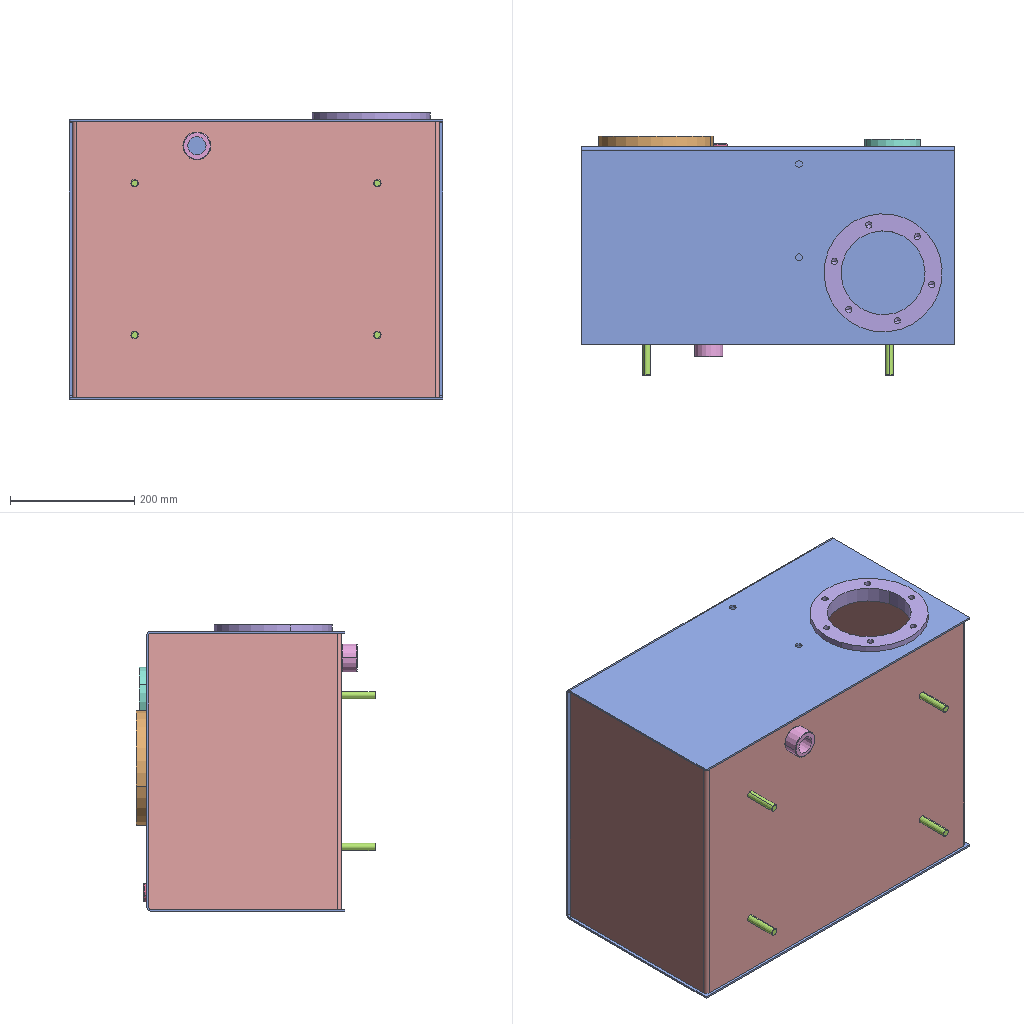Assembly | SolidWorks | 10 different items | 19 placed | box 600 x 385 x 460 mm
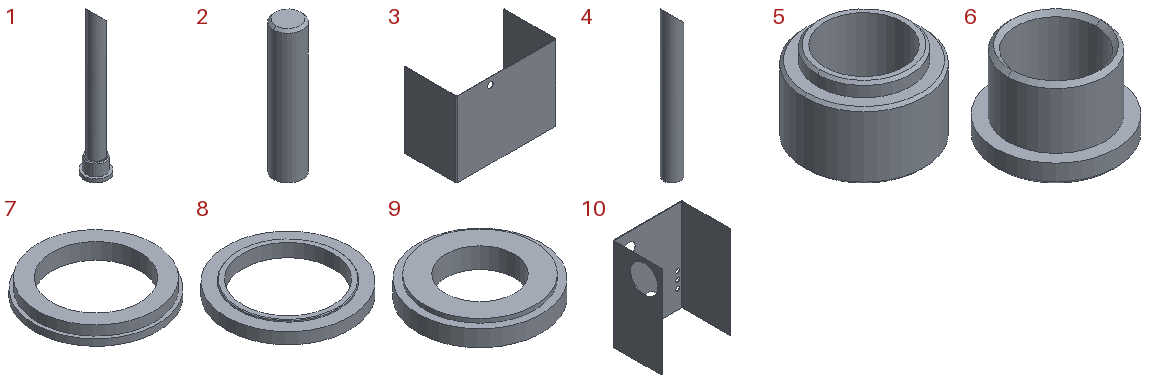Parts list (item | name | quantity | parent item | size | volume | features):
1 | (subassembly) | x3 | - | 30 x 30 x 180 mm | 11987 mm3 | features CompositeCurve 2, AEMSimFeature 1
2 | - | x4 | - | 12 x 12 x 55 mm | 6203 mm3 | features Chamfer 1, Extrusion 1
3 | - | x1 | - | 590 x 310 x 444 mm | 1595673 mm3 | features ICE 2, FlatPattern 1, SMBaseFlange 1, SheetMetal 1
4 | - | x3 | in 1 | 18 x 18 x 160 mm | 8065 mm3 | features Extrusion 1, ICE 1
5 | - | x1 | - | 45 x 45 x 30 mm | 23873 mm3 | features Chamfer 1, Extrusion 1, ICE 1
6 | - | x3 | in 1 | 30 x 30 x 20 mm | 3922 mm3 | features Chamfer 1, Extrusion 1, ICE 1
7 | - | x1 | - | 190 x 190 x 25 mm | 301982 mm3 | features 3DProfileFeature 1, Extrusion 1, HoleWzd 1, ICE 1
8 | - | x1 | - | 185 x 185 x 20 mm | 216002 mm3 | features Fillet 2, ICE 2, 3DProfileFeature 1, Chamfer 1, Extrusion 1, HoleWzd 1
9 | - | x1 | - | 90 x 90 x 15 mm | 61433 mm3 | features 3DProfileFeature 1, Extrusion 1, HoleWzd 1, ICE 1
10 | - | x1 | - | 450 x 318 x 600 mm | 1787947 mm3 | features ICE 3, FlatPattern 1, SMBaseFlange 1, SheetMetal 1
Mates (type | each side: item.copy, entity, surface, feature):
In the top assembly
Coincident | 3.1 face plane Base-Flange1 | 10.1 face plane Base-Flange1 | 2 times
DistanceDim | 10.1 face plane Base-Flange1 | 3.1 face plane Base-Flange1
Concentric | 2.1 edge | assembly select_type:10
Coincident | 3.1 face plane Base-Flange1 | 2.1 face plane Boss-Extrude1
Coincident | 2.1 face plane Boss-Extrude1 | 2.2 face plane Boss-Extrude1
Coincident | 2.3 face plane Boss-Extrude1 | 2.2 face plane Boss-Extrude1
Coincident | 2.4 face plane Boss-Extrude1 | 2.2 face plane Boss-Extrude1
Concentric | 2.2 edge | assembly select_type:10
Concentric | 2.4 edge | assembly select_type:10
Concentric | 2.3 edge | assembly select_type:10
Concentric | 3.1 edge | 5.1 edge
Coincident | 3.1 face plane Base-Flange1 | 5.1 face plane Boss-Extrude1
Coincident | 10.1 face plane Base-Flange1 | 9.1 face plane Boss-Extrude1
Concentric | 10.1 edge | 9.1 edge
Coincident | 10.1 face plane Base-Flange1 | 8.1 face plane Boss-Extrude1
Concentric | 10.1 edge | 8.1 edge
Coincident | 10.1 face plane Base-Flange1 | 7.1 face plane Boss-Extrude1
Concentric | 10.1 edge | 7.1 edge
Coincident | 10.1 face plane Base-Flange1 | 6.1 face plane Boss-Extrude1
Concentric | 10.1 edge | 6.1 edge
Coincident | 6.1 face plane Boss-Extrude1 | 6.2 face plane Boss-Extrude1
Coincident | 6.1 face plane Boss-Extrude1 | 6.3 face plane Boss-Extrude1
Concentric | 10.1 edge | 6.3 edge
Concentric | 10.1 edge | 6.2 edge
In subassembly 1
Concentric | 4.1 edge | 6.4 edge
DistanceDim | 4.1 face plane Boss-Extrude1 | 6.4 face plane Boss-Extrude1